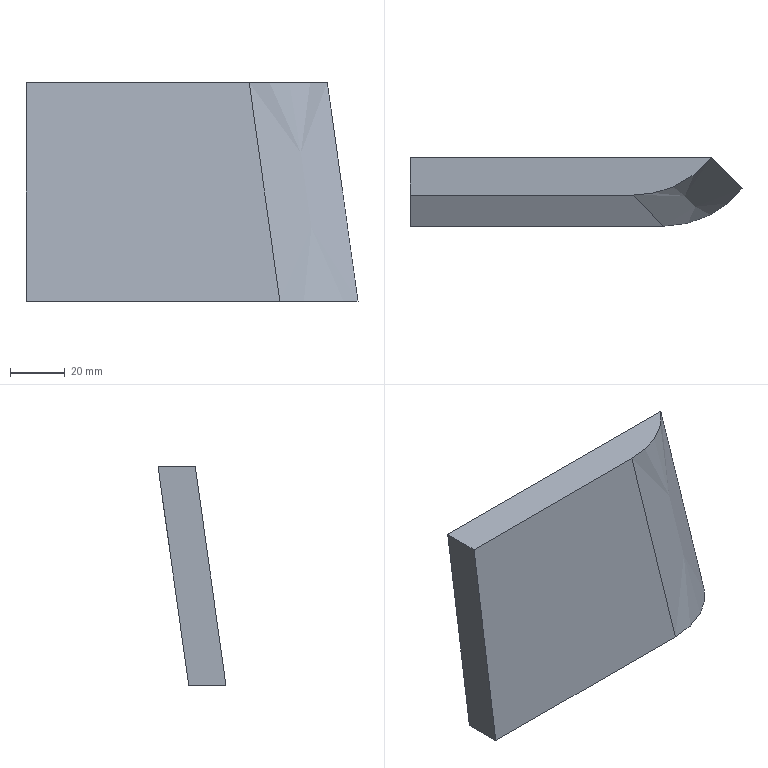Part | STEP file | solid 22 | 1 solid | 6 faces | box 121.532 x 24.876 x 80 mm | volume 116975 mm3 | spline 6